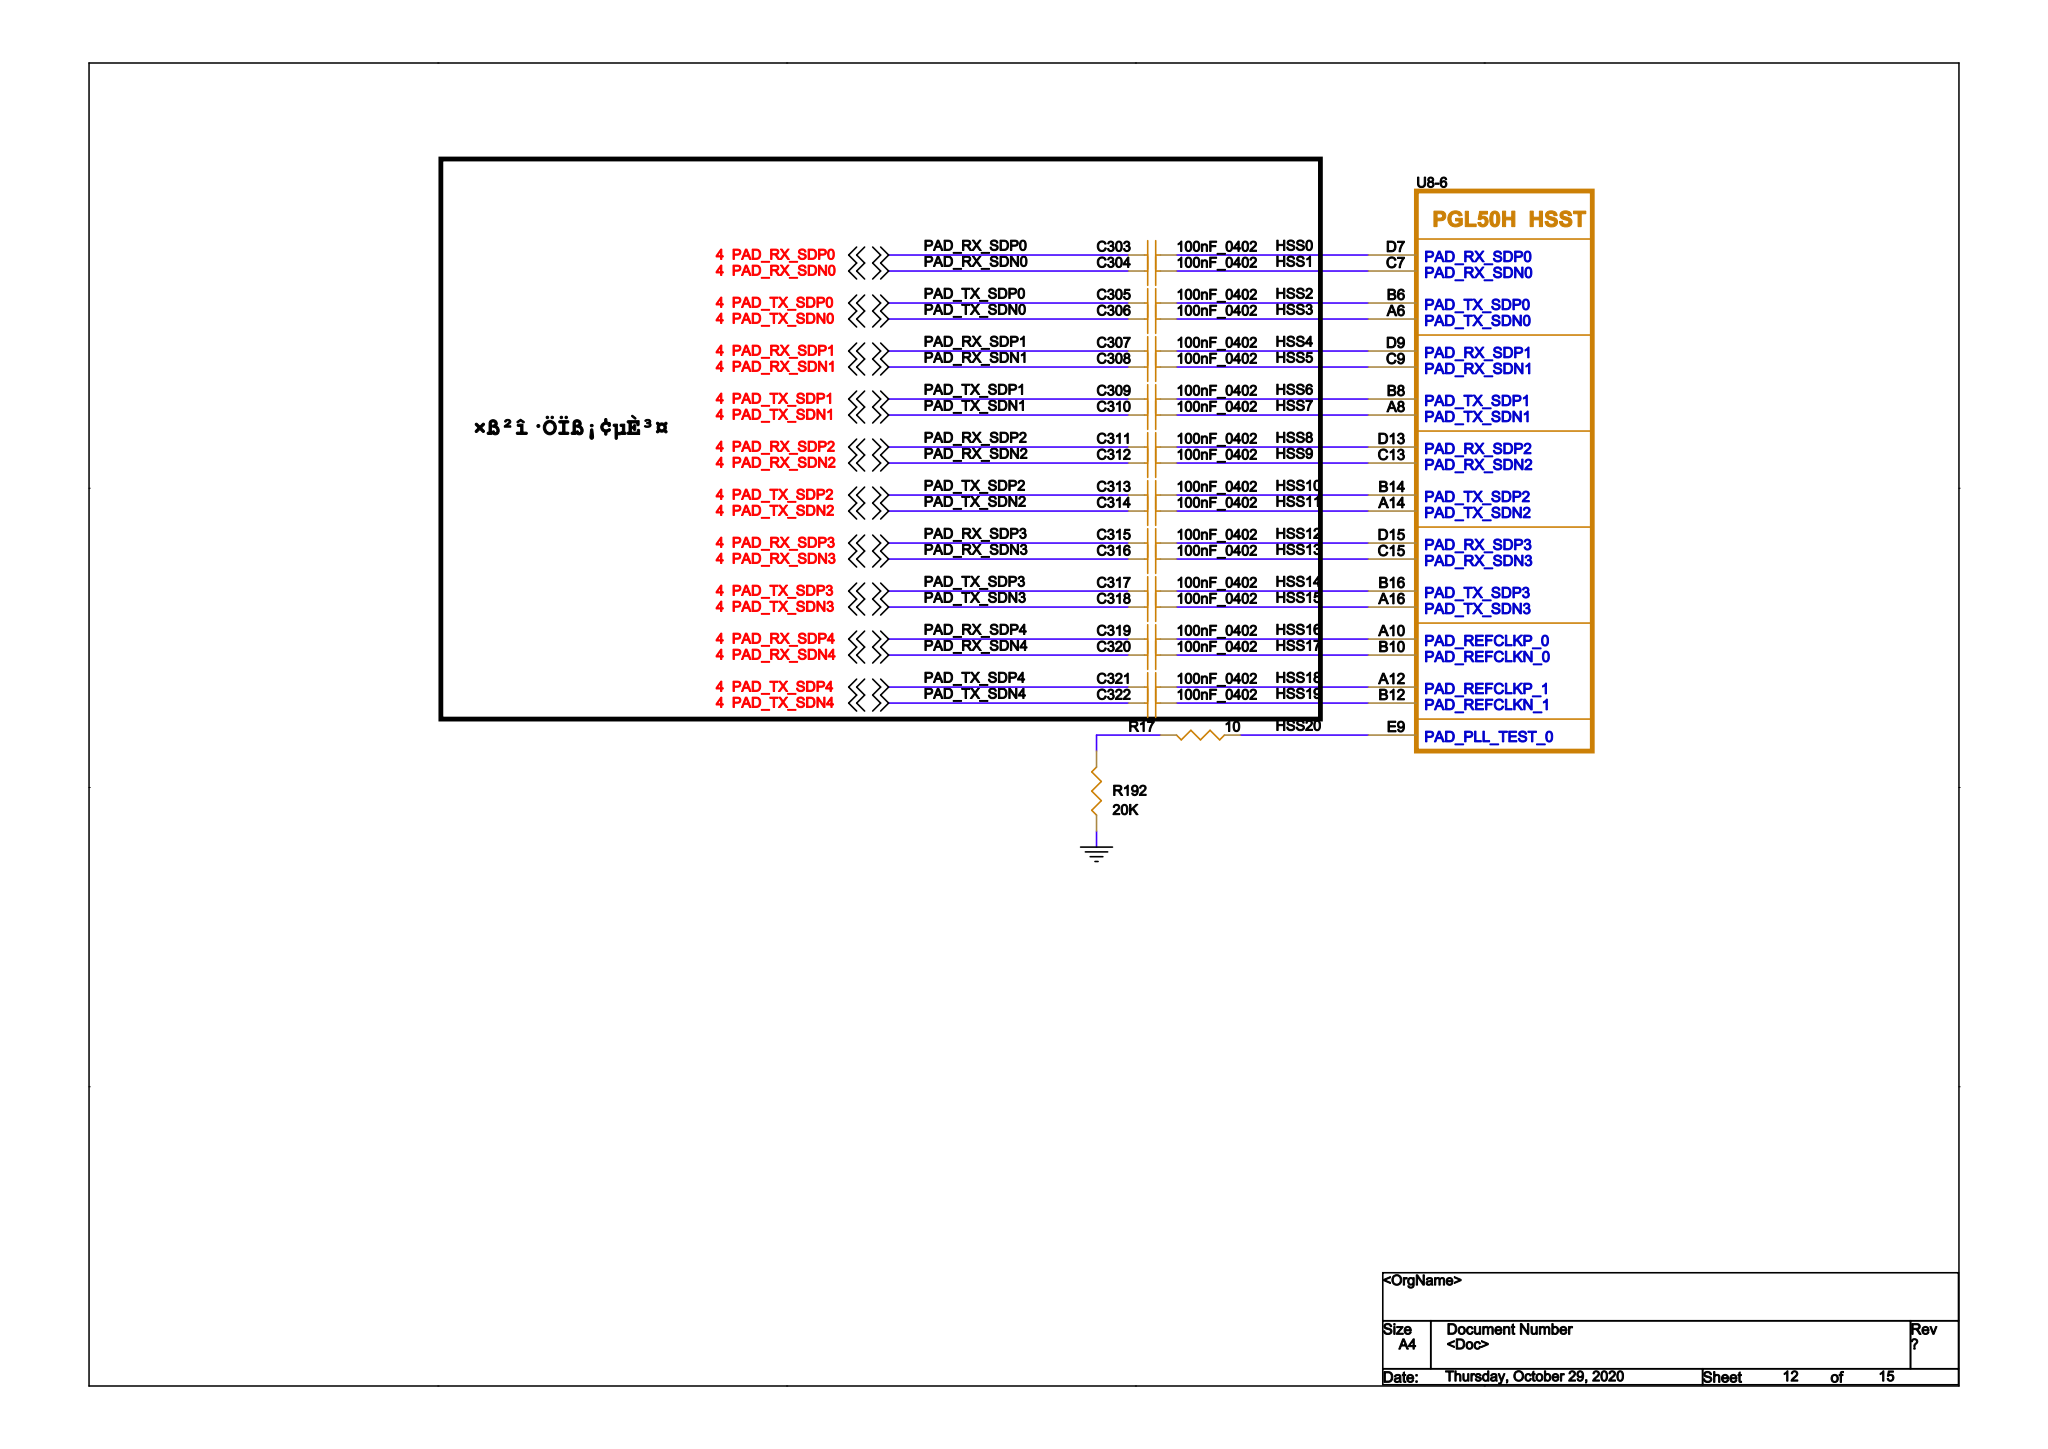Circuit board | Cadence Allegro | 406 parts | 392 nets | one sheet of the schematic
Parts on this sheet (reference | value | footprint):
C303 | 100nF_0402 | C_0402_104
C304 | 100nF_0402 | C_0402_104
C305 | 100nF_0402 | C_0402_104
C306 | 100nF_0402 | C_0402_104
C307 | 100nF_0402 | C_0402_104
C308 | 100nF_0402 | C_0402_104
C309 | 100nF_0402 | C_0402_104
C310 | 100nF_0402 | C_0402_104
C311 | 100nF_0402 | C_0402_104
C312 | 100nF_0402 | C_0402_104
C313 | 100nF_0402 | C_0402_104
C314 | 100nF_0402 | C_0402_104
C315 | 100nF_0402 | C_0402_104
C316 | 100nF_0402 | C_0402_104
C317 | 100nF_0402 | C_0402_104
C318 | 100nF_0402 | C_0402_104
C319 | 100nF_0402 | C_0402_104
C320 | 100nF_0402 | C_0402_104
C321 | 100nF_0402 | C_0402_104
C322 | 100nF_0402 | C_0402_104
R17 | 10 | R_0603
R192 | 20K | R_0603
Nets of these parts (net: part-pin ...):
GND: R192-1
PAD_RX_SDP0: C303-1
PAD_RX_SDN0: C304-1
PAD_RX_SDP1: C307-1
PAD_RX_SDN1: C308-1
PAD_RX_SDP2: C311-1
PAD_RX_SDN2: C312-1
PAD_RX_SDP3: C315-1
PAD_RX_SDN3: C316-1
PAD_RX_SDP4: C319-1
PAD_RX_SDN4: C320-1
PAD_TX_SDP0: C305-1
PAD_TX_SDN0: C306-1
PAD_TX_SDP1: C309-1
PAD_TX_SDN1: C310-1
PAD_TX_SDP2: C313-1
PAD_TX_SDN2: C314-1
PAD_TX_SDP3: C317-1
PAD_TX_SDN3: C318-1
PAD_TX_SDP4: C321-1
PAD_TX_SDN4: C322-1
HSS0: C303-2
HSS1: C304-2
HSS2: C305-2
HSS3: C306-2
HSS4: C307-2
HSS5: C308-2
HSS6: C309-2
HSS7: C310-2
HSS8: C311-2
HSS9: C312-2
HSS10: C313-2
HSS11: C314-2
HSS12: C315-2
HSS13: C316-2
HSS14: C317-2
HSS15: C318-2
HSS16: C319-2
HSS17: C320-2
HSS18: C321-2
HSS19: C322-2
HSS20: R17-1
N20090611: R17-2 R192-2